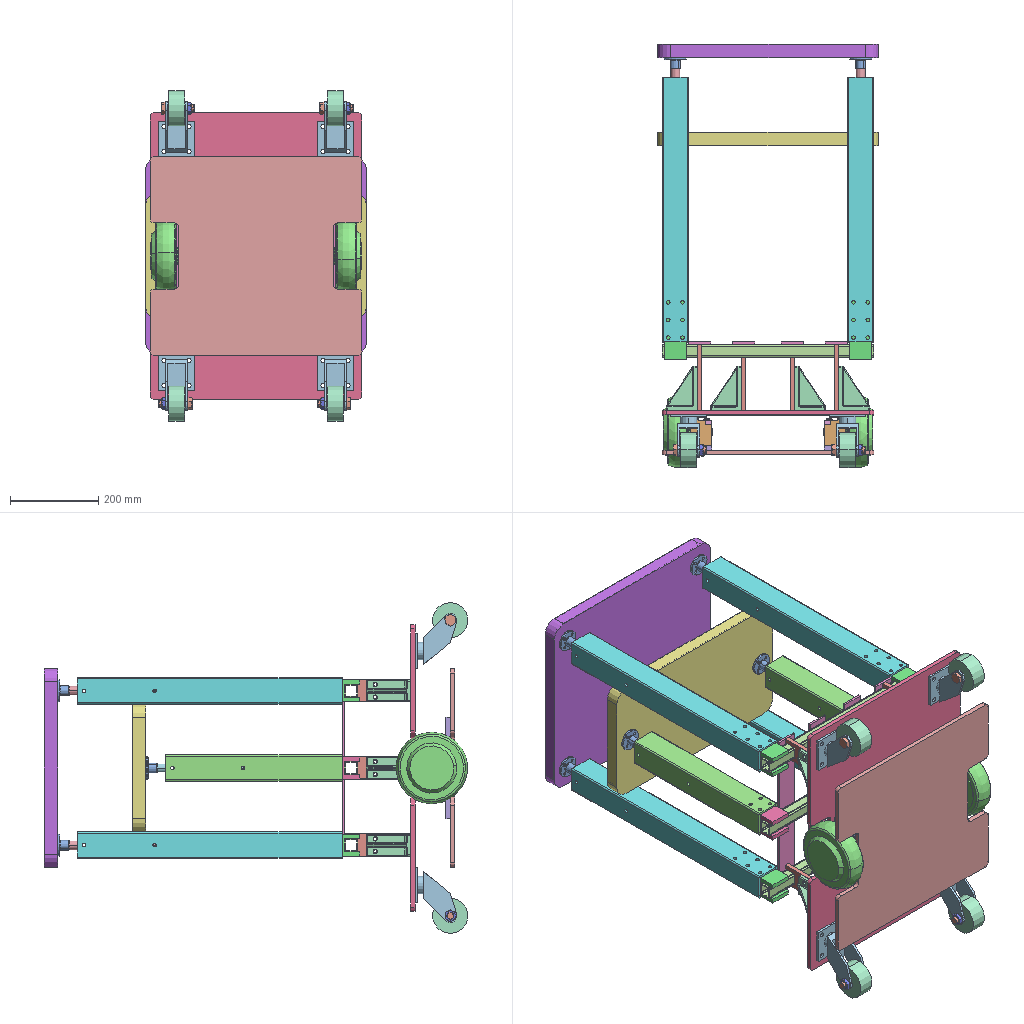Assembly | SolidWorks | 41 different items | 214 placed | box 500 x 959 x 750 mm
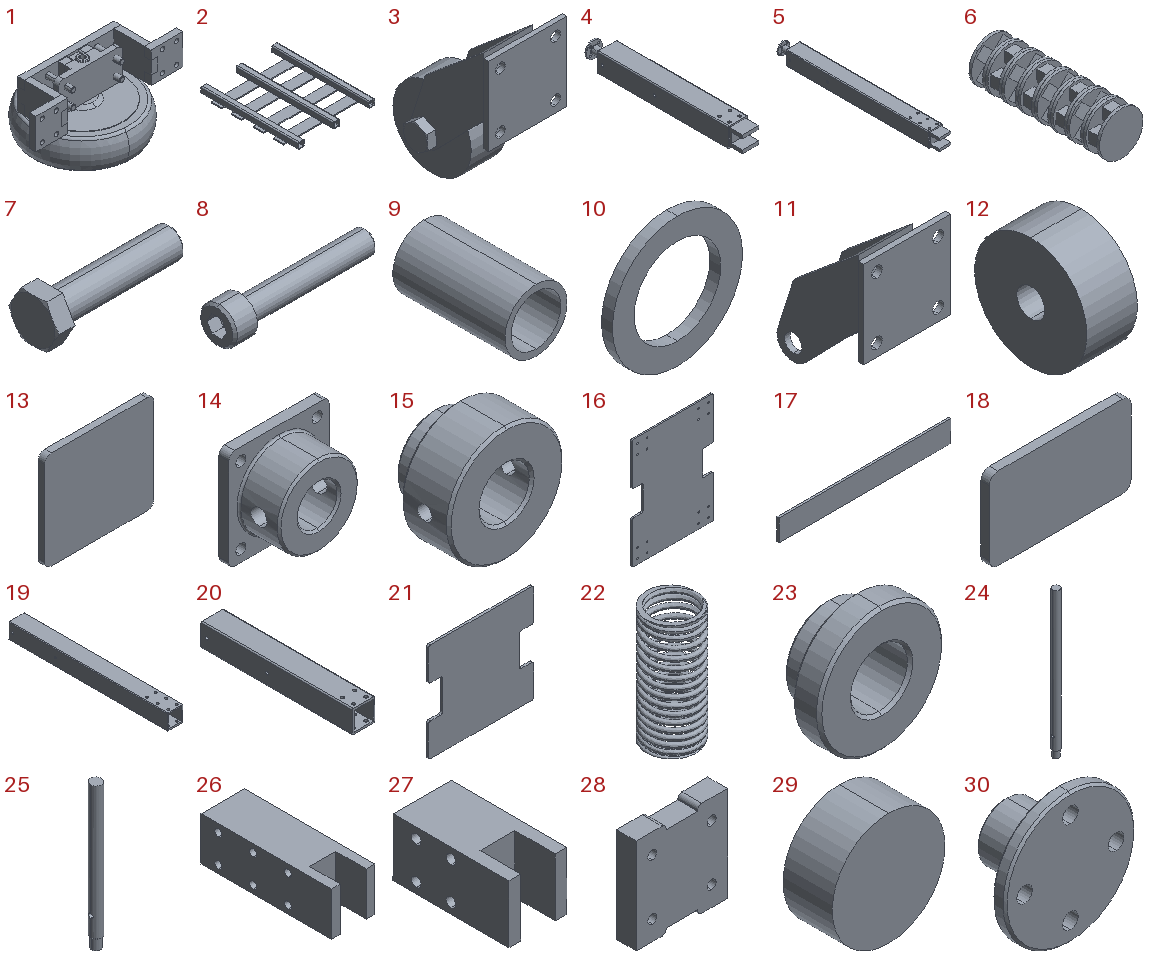Parts list (item | name | quantity | parent item | size | volume | features):
1 | (subassembly) | x2 | - | 230 x 163 x 112 mm | 1242773 mm3 | -
2 | (subassembly) | x1 | - | 400 x 480 x 35 mm | 772823 mm3 | -
3 | (subassembly) | x4 | - | 80 x 120 x 150 mm | 311923 mm3 | features CompositeCurve 1
4 | (subassembly) | x2 | - | 60 x 485 x 60 mm | 1102301 mm3 | -
5 | (subassembly) | x4 | - | 60 x 685 x 60 mm | 1570398 mm3 | -
6 | (subassembly) | x6 | in 4, 5 | 32 x 96 x 32 mm | 42120 mm3 | -
7 | - | x4 | in 3 | 75 x 27.713 x 24 mm | 17960 mm3 | features RevCut 3, Boss 1, Chamfer 1, Extrusion 1, Fillet 1, LPattern 1
8 | - | x8 | in 1 | 53 x 13 x 13 mm | 3161 mm3 | features CirPattern 3, Cut 3, RevCut 2, Fillet 1, LPattern 1, Revolution 1
9 | - | x4 | in 3 | 20 x 36 x 20 mm | 4072 mm3 | features Extrusion 1
10 | - | x8 | in 3 | 24 x 2 x 24 mm | 502.655 mm3 | features Extrusion 1
11 | - | x4 | in 3 | 80 x 95 x 125 mm | 116525 mm3 | features ICE 3, Extrusion 1
12 | - | x4 | in 3 | 36 x 80 x 80 mm | 169646 mm3 | features Revolution 1
13 | - | x1 | - | 500 x 30 x 450 mm | 1262737 mm3 | features Extrusion 1, ICE 1
14 | - | x6 | in 4, 5 | 50 x 25 x 50 mm | 28265 mm3 | features ICE 4, Fillet 2, Chamfer 1, Extrusion 1
15 | - | x6 | in 4, 5 | 48 x 30 x 48 mm | 32861 mm3 | features ICE 3, Chamfer 2, Extrusion 1
16 | - | x1 | - | 480 x 10 x 650 mm | 2911575 mm3 | features Fillet 2, ICE 2, Extrusion 1
17 | - | x4 | in 2 | 400 x 5 x 50 mm | 100000 mm3 | features Extrusion 1
18 | - | x1 | - | 500 x 30 x 290 mm | 838737 mm3 | features Extrusion 1, ICE 1
19 | - | x4 | in 5 | 60 x 600 x 60 mm | 948372 mm3 | features ICE 9, Fillet 2, Extrusion 1
20 | - | x2 | in 4 | 60 x 400 x 60 mm | 650447 mm3 | features ICE 9, Fillet 2, Extrusion 1
21 | - | x1 | - | 480 x 10 x 450 mm | 1964142 mm3 | features Fillet 2, ICE 2, Extrusion 1
22 | - | x6 | in 4, 5 | - | 25238 mm3 | features Helix 1, ICE 1, Sweep 1
23 | - | x6 | in 4, 5 | 46 x 20 x 46 mm | 17526 mm3 | features Chamfer 2, ICE 2, Extrusion 1
24 | - | x4 | in 5 | 20 x 20 x 410 mm | 125504 mm3 | features ICE 4, Chamfer 1, Revolution 1
25 | - | x2 | in 4 | 20 x 20 x 260 mm | 78380 mm3 | features ICE 4, Chamfer 2, Revolution 1
26 | - | x4 | in 5 | 50 x 150 x 50 mm | 308426 mm3 | features ICE 3, Extrusion 1, MirrorPattern 1
27 | - | x2 | in 4 | 50 x 100 x 50 mm | 185436 mm3 | features ICE 4, Extrusion 1
28 | - | x2 | in 1 | 46 x 10 x 48 mm | 19482 mm3 | features ICE 2, Extrusion 1, Fillet 1, HoleWzd 1
29 | - | x6 | in 4, 5 | 32 x 14 x 32 mm | 11259 mm3 | features Extrusion 1
30 | - | x6 | in 4, 5 | 50 x 25 x 50 mm | 12711 mm3 | features ICE 2, Chamfer 1, Extrusion 1, Fillet 1
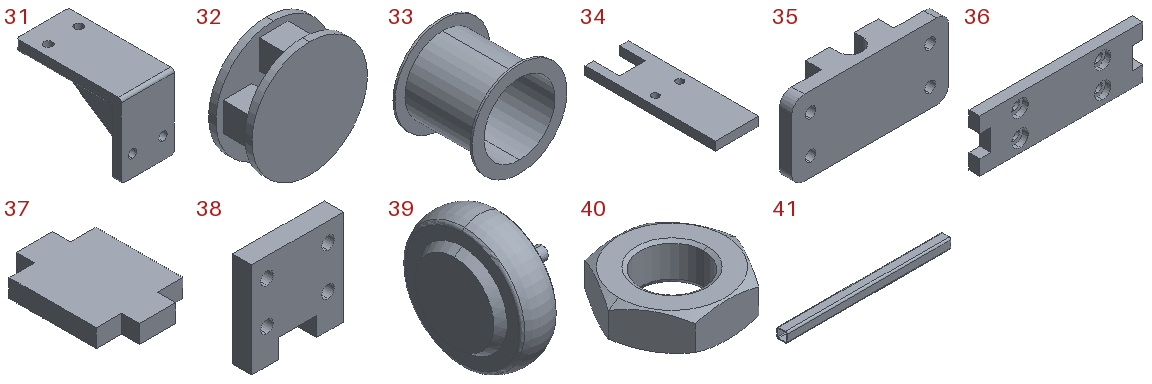31 | - | x6 | - | 50 x 100 x 70 mm | 99196 mm3 | features Fillet 5, ICE 3, MirrorPattern 2, Chamfer 1, Extrusion 1
32 | - | x48 | in 6 | 32 x 12 x 32 mm | 5265 mm3 | features ICE 2, Extrusion 1
33 | - | x18 | in 4, 5 | 48 x 40 x 48 mm | 6000 mm3 | features Revolution 1
34 | - | x6 | - | 50 x 150 x 10 mm | 64995 mm3 | features ICE 2, Extrusion 1
35 | - | x2 | in 1 | 100 x 18 x 48 mm | 49859 mm3 | features HoleWzd 2, ICE 2, Extrusion 1, Fillet 1
36 | - | x2 | in 1 | 150 x 10 x 48 mm | 62310 mm3 | features ICE 2, Extrusion 1, HoleWzd 1
37 | - | x4 | in 1 | 48 x 68 x 10 mm | 27040 mm3 | features Extrusion 1, ICE 1
38 | - | x4 | in 1 | 48 x 10 x 50 mm | 19683 mm3 | features Extrusion 1, HoleWzd 1, ICE 1
39 | - | x2 | in 1 | 112 x 163 x 163 mm | 1005033 mm3 | features ICE 2, Chamfer 1, Fillet 1, Revolution 1
40 | - | x4 | in 3 | 27.713 x 24 x 8 mm | 2715 mm3 | features RevCut 2, Chamfer 1, Extrusion 1, LPattern 1
41 | - | x3 | in 2 | 480 x 30 x 30 mm | 124274 mm3 | features WeldMemberFeat 1, WeldmentFeature 1
Mates (type | each side: item.copy, entity, surface, feature):
In the top assembly
Coincident | 21.1 face plane Boss-Extrude1 | 38.1 face plane Boss-Extrude1
Coincident | 21.1 face plane Boss-Extrude1 | 38.2 face plane Boss-Extrude1
Coincident | 21.1 face plane Boss-Extrude1 | 38.3 face plane Boss-Extrude1
Coincident | 21.1 face plane Boss-Extrude1 | 38.4 face plane Boss-Extrude1
Coincident | 21.1 face plane Boss-Extrude1 | 16.1 face plane Boss-Extrude1
DistanceDim | 16.1 face plane Boss-Extrude1 | 21.1 face plane Boss-Extrude1
Coincident | 16.1 face plane Boss-Extrude1 | 11.1 face plane Boss-Extrude3
DistanceDim | 11.1 face plane Boss-Extrude3 | 16.1 face plane Boss-Extrude1 | 2 times
Coincident | 16.1 face plane Boss-Extrude1 | 11.2 face plane Boss-Extrude3
Coincident | 11.1 face plane Boss-Extrude3 | 11.2 face plane Boss-Extrude3
DistanceDim | 11.2 face plane Boss-Extrude3 | 16.1 face plane Boss-Extrude1
Coincident | 16.1 face plane Boss-Extrude1 | 11.3 face plane Boss-Extrude3
Coincident | 11.2 face plane Boss-Extrude3 | 11.3 face plane Boss-Extrude3
DistanceDim | 11.3 face plane Boss-Extrude3 | 16.1 face plane Boss-Extrude1
Coincident | 16.1 face plane Boss-Extrude1 | 11.4 face plane Boss-Extrude3
Coincident | 11.3 face plane Boss-Extrude3 | 11.4 face plane Boss-Extrude3
Coincident | 11.1 face plane Boss-Extrude3 | 11.4 face plane Boss-Extrude3
Coincident | 16.1 face plane Boss-Extrude1 | assembly face
Parallel | 16.1 face plane Boss-Extrude1 | assembly face | 2 times
DistanceDim | assembly face | 16.1 face plane Boss-Extrude1 | 2 times
Coincident | 41.1 face plane Square tube 30 X 30 X 2.5 | 26.1 face plane Cut-Extrude1 | 2 times
Coincident | 41.1 face plane Square tube 30 X 30 X 2.5 | 26.2 face plane Cut-Extrude1 | 2 times
Coincident | 41.2 face plane Square tube 30 X 30 X 2.5 | 26.3 face plane Cut-Extrude1 | 2 times
Coincident | 41.2 face plane Square tube 30 X 30 X 2.5 | 26.4 face plane Cut-Extrude1 | 2 times
DistanceDim | 26.2 face plane Boss-Extrude2 | 41.1 face plane Square tube 30 X 30 X 2.5
DistanceDim | 26.3 face plane Boss-Extrude2 | 41.2 face plane Square tube 30 X 30 X 2.5
DistanceDim | 26.4 face plane Boss-Extrude2 | 41.2 face plane Square tube 30 X 30 X 2.5
DistanceDim | 26.1 face plane Boss-Extrude2 | 41.1 face plane Square tube 30 X 30 X 2.5
Coincident | 41.3 face plane Square tube 30 X 30 X 2.5 | 27.1 face plane Cut-Extrude2 | 2 times
Coincident | 41.3 face plane Square tube 30 X 30 X 2.5 | 27.2 face plane Cut-Extrude2 | 2 times
DistanceDim | 27.2 face plane Boss-Extrude1 | 41.3 face plane Square tube 30 X 30 X 2.5
DistanceDim | 27.1 face plane Boss-Extrude1 | 41.3 face plane Square tube 30 X 30 X 2.5
Coincident | 19.1 face plane Boss-Extrude1 | 18.1 face plane Boss-Extrude1
Coincident | 30.1 face plane Boss-Extrude2 | 18.1 face plane Boss-Extrude1
DistanceDim | 18.1 face plane Boss-Extrude1 | 19.2 face plane Boss-Extrude1
Coincident | 30.2 face plane Boss-Extrude2 | 13.1 face plane Boss-Extrude1
DistanceDim | 13.1 face plane Boss-Extrude1 | 19.3 face plane Boss-Extrude1 | 2 times
DistanceDim | 21.1 face plane Cut-Extrude2 | 16.1 face plane Boss-Extrude1
Coincident | 21.1 face plane Cut-Extrude1 | 38.3 face plane Boss-Extrude1
Coincident | 21.1 face plane Cut-Extrude1 | 37.1 face plane Boss-Extrude1
Coincident | 21.1 face plane Cut-Extrude1 | 38.1 face plane Boss-Extrude1
Coincident | 21.1 face plane Cut-Extrude1 | 37.2 face plane Boss-Extrude1
Coincident | assembly face | 31.1 face plane Boss-Extrude1 | 2 times
Coincident | assembly face | 31.2 face plane Boss-Extrude1 | 2 times
Coincident | assembly face | 31.3 face plane Boss-Extrude1 | 2 times
Coincident | assembly face | 31.4 face plane Boss-Extrude1 | 2 times
Coincident | assembly face | 31.5 face plane Boss-Extrude1 | 2 times
Coincident | assembly face | 31.6 face plane Boss-Extrude1 | 2 times
Coincident | 31.1 face plane Boss-Extrude1 | 34.1 face plane Boss-Extrude1
Width | 31.1 face plane Boss-Extrude1 | 31.1 face plane Boss-Extrude1 | 34.1 face plane Boss-Extrude1 | 34.1 face plane Boss-Extrude1
Coincident | 16.1 face plane Boss-Extrude1 | 34.1 face plane Boss-Extrude1
Coincident | 31.4 face plane Boss-Extrude1 | 34.2 face plane Boss-Extrude1
Concentric | 31.4 face cylinder Mirror1 | 34.2 face cylinder Cut-Extrude2
Parallel | 31.4 face plane Boss-Extrude1 | 34.2 face plane Boss-Extrude1
Coincident | 31.5 face plane Boss-Extrude1 | 34.3 face plane Boss-Extrude1
Concentric | 31.5 face cylinder Mirror1 | 34.3 face cylinder Cut-Extrude2
Parallel | 31.5 face plane Boss-Extrude1 | 34.3 face plane Boss-Extrude1
Coincident | 31.6 face plane Boss-Extrude1 | 34.4 face plane Boss-Extrude1
Concentric | 31.6 face cylinder Mirror1 | 34.4 face cylinder Cut-Extrude2
Parallel | 31.6 face plane Boss-Extrude1 | 34.4 face plane Boss-Extrude1
Concentric | 31.2 face cylinder Mirror1 | 34.5 face cylinder Cut-Extrude2
Parallel | 31.2 face plane Boss-Extrude1 | 34.5 face plane Boss-Extrude1
Coincident | 31.3 face plane Boss-Extrude1 | 34.6 face plane Boss-Extrude1
Concentric | 31.3 face cylinder Mirror1 | 34.6 face cylinder Cut-Extrude2
Parallel | 31.3 face plane Boss-Extrude1 | 34.6 face plane Boss-Extrude1
In subassembly 4
Coincident | 20.1 face plane Cut-Extrude1 | 14.1 face plane Boss-Extrude3
Concentric | 20.1 face cylinder Cut-Extrude4 | 14.1 face cylinder Cut-Extrude5
Concentric | 20.1 face cylinder Cut-Extrude2 | 14.1 face cylinder Cut-Extrude6
Coincident | 20.1 face plane Cut-Extrude5 | 33.1 face plane Revolve2
Concentric | 20.1 face cylinder Cut-Extrude6 | 33.1 face cylinder Revolve2
Coincident | 20.1 face plane Cut-Extrude5 | 27.3 face plane Boss-Extrude1 | 3 times
Concentric | 14.1 face cylinder Cut-Extrude6 | 25.1 face cylinder Revolve4
Concentric | 20.1 face cylinder Cut-Extrude4 | 25.1 face cylinder Cut-Extrude1
DistanceDim | 23.1 face plane Boss-Extrude1 | 15.1 face plane Boss-Extrude1
Coincident | 22.1 face plane Cut-Extrude1 | 23.1 face plane Boss-Extrude1
Concentric | 33.1 face cylinder Revolve2 | 33.2 face cylinder Revolve2
Coincident | 33.1 face plane Revolve2 | 33.2 face plane Revolve2
Concentric | 25.1 face cylinder Revolve4 | 33.3 face cylinder Revolve2
Coincident | 33.2 face plane Revolve2 | 33.3 face plane Revolve2
Coincident | 25.1 face plane Boss-Extrude3 | 32.1 face plane Boss-Extrude8
Concentric | 25.1 face cylinder Revolve4 | 32.1 face cylinder Boss-Extrude8
Parallel | 27.3 face plane Boss-Extrude1 | 32.2 face plane Boss-Extrude7
Concentric | 23.1 face cylinder Boss-Extrude1 | 15.1 face cylinder Boss-Extrude1
Concentric | 25.1 face cylinder Revolve4 | 15.1 face cylinder Cut-Extrude3
Concentric | 20.1 face cylinder Cut-Extrude7 | 15.1 face cylinder Cut-Extrude2
Concentric | 25.1 face cylinder Boss-Extrude5 | 30.3 face cylinder Boss-Extrude3
Coincident | 25.1 face plane Boss-Extrude4 | 30.3 face plane Boss-Extrude3
Coincident | 27.3 face plane Cut-Extrude3 | 29.1 face plane Boss-Extrude1
Concentric | 27.3 face cylinder Cut-Extrude3 | 29.1 face cylinder Boss-Extrude1
In subassembly 6
Coincident | 32.3 face plane Boss-Extrude8 | 32.4 face plane Boss-Extrude2
Concentric | 32.3 face cylinder Boss-Extrude8 | 32.4 face cylinder Boss-Extrude2
Concentric | 32.3 face cylinder Boss-Extrude8 | 32.5 face cylinder Boss-Extrude2
Coincident | 32.4 face plane Boss-Extrude8 | 32.5 face plane Boss-Extrude2
Coincident | 32.6 face plane Boss-Extrude2 | 32.5 face plane Boss-Extrude8
Concentric | 32.6 face cylinder Boss-Extrude2 | 32.5 face cylinder Boss-Extrude8
Coincident | 32.7 face plane Boss-Extrude8 | 32.8 face plane Boss-Extrude2
Concentric | 32.7 face cylinder Boss-Extrude8 | 32.8 face cylinder Boss-Extrude2
Coincident | 32.7 face plane Boss-Extrude2 | 32.6 face plane Boss-Extrude8
Concentric | 32.7 face cylinder Boss-Extrude2 | 32.6 face cylinder Boss-Extrude8
Coincident | 32.9 face plane Boss-Extrude2 | 32.10 face plane Boss-Extrude8 | 2 times
Concentric | 32.9 face cylinder Boss-Extrude2 | 32.10 face cylinder Boss-Extrude8
Coincident | 32.10 face plane Boss-Extrude2 | 32.8 face plane Boss-Extrude8
Concentric | 32.10 face cylinder Boss-Extrude2 | 32.8 face cylinder Boss-Extrude8
PlanarAngleDim | 32.4 face plane Boss-Extrude7 | 32.3 face plane Boss-Extrude7
Coincident | 32.3 face plane Boss-Extrude7 | 32.5 face plane Boss-Extrude7
Coincident | 32.7 face plane Boss-Extrude7 | 32.5 face plane Boss-Extrude7
Coincident | 32.4 face plane Boss-Extrude7 | 32.6 face plane Boss-Extrude7
Coincident | 32.6 face plane Boss-Extrude7 | 32.8 face plane Boss-Extrude7
Coincident | 32.10 face plane Boss-Extrude7 | 32.7 face plane Boss-Extrude7
Coincident | 32.9 face plane Boss-Extrude7 | 32.8 face plane Boss-Extrude7
In subassembly 3
Concentric | 9.1 face cylinder Boss-Extrude1 | 12.1 face cylinder Revolve1
Coincident | 9.1 face plane Boss-Extrude1 | 12.1 face plane Revolve1
Coincident | 10.1 edge | 12.1 face plane Revolve1
Concentric | 9.1 face cylinder Boss-Extrude1 | 10.1 face cylinder Boss-Extrude3
Coincident | 10.2 face plane Boss-Extrude3 | 12.1 face plane Revolve1
Concentric | 9.1 face cylinder Boss-Extrude1 | 10.2 face cylinder Boss-Extrude3
Concentric | 11.5 face cylinder Boss-Extrude6 | 9.1 face cylinder Boss-Extrude1
Coincident | 11.5 face plane Cut-Extrude1 | 10.1 face plane Boss-Extrude3
Concentric | 9.1 face cylinder Boss-Extrude1 | 7.1 face cylinder BaseBody
Coincident | 11.5 face plane Boss-Extrude6 | 7.1 face plane BaseHead
Concentric | 7.1 face cylinder BaseBody | 40.1 face cylinder BaseNut
Coincident | 11.5 face plane Boss-Extrude6 | 40.1 face plane BaseNut
In subassembly 5
Concentric | 19.4 face cylinder Cut-Extrude7 | 14.1 face cylinder Cut-Extrude6
Concentric | 19.4 face cylinder Cut-Extrude3 | 14.1 face cylinder Cut-Extrude5
Concentric | 19.4 face cylinder Cut-Extrude6 | 33.1 face cylinder Revolve2
Coincident | 19.4 face plane Cut-Extrude5 | 33.1 face plane Revolve2
Coincident | 19.4 face plane Cut-Extrude5 | 26.5 face plane Boss-Extrude2 | 3 times
Coincident | 19.4 face plane Cut-Extrude5 | 26.5 select_type:24
Concentric | 14.1 face cylinder Cut-Extrude6 | 24.1 face cylinder Revolve4
Concentric | 19.4 face cylinder Cut-Extrude3 | 24.1 face cylinder Cut-Extrude1
Concentric | 15.1 face cylinder Cut-Extrude3 | 23.1 face cylinder Cut-Extrude1
Coincident | 22.2 face plane Cut-Extrude1 | 23.1 face plane Boss-Extrude1
Coincident | 22.2 face plane Cut-Extrude1 | 15.1 face plane Boss-Extrude1
Concentric | 24.1 face cylinder Boss-Extrude2 | 30.3 face cylinder Boss-Extrude3
Coincident | 24.1 face plane Boss-Extrude1 | 30.3 face plane Boss-Extrude3
Concentric | 19.4 face cylinder Cut-Extrude8 | 15.1 face cylinder Cut-Extrude2
Concentric | 24.1 face cylinder Revolve4 | 23.1 face cylinder Cut-Extrude1
Coincident | 33.2 face plane Revolve2 | 33.3 face plane Revolve2
Concentric | 33.2 face cylinder Revolve2 | 33.3 face cylinder Revolve2
Concentric | 33.1 face cylinder Revolve2 | 33.2 face cylinder Revolve2
Coincident | 33.1 face plane Revolve2 | 33.2 face plane Revolve2
Coincident | 24.1 face plane Boss-Extrude4 | 32.1 face plane Boss-Extrude8
Concentric | 24.1 face cylinder Revolve4 | 32.1 face cylinder Boss-Extrude8
Parallel | 26.5 face plane Boss-Extrude2 | 32.11 face plane Boss-Extrude7
Coincident | 26.5 face plane Cut-Extrude2 | 29.1 face plane Boss-Extrude1
Concentric | 26.5 face cylinder Cut-Extrude2 | 29.1 face cylinder Boss-Extrude1
In subassembly 2
Width | 2.1 face | 2.1 face | 41.4 face plane Square tube 30 X 30 X 2.5 | 41.4 face plane Square tube 30 X 30 X 2.5
DistanceDim | 41.4 face plane Square tube 30 X 30 X 2.5 | 2.1 face
Coincident | 41.4 face plane Square tube 30 X 30 X 2.5 | 2.1 face
DistanceDim | 41.4 face plane Square tube 30 X 30 X 2.5 | 17.1 face plane Boss-Extrude1
Coincident | 41.4 face plane Square tube 30 X 30 X 2.5 | 17.1 face plane Boss-Extrude1
DistanceDim | 41.5 face plane Square tube 30 X 30 X 2.5 | 17.1 face plane Boss-Extrude1
Coincident | 17.1 face plane Boss-Extrude1 | 41.5 face plane Square tube 30 X 30 X 2.5
DistanceDim | 41.6 face plane Square tube 30 X 30 X 2.5 | 41.4 face plane Square tube 30 X 30 X 2.5
Coincident | 41.6 face plane Square tube 30 X 30 X 2.5 | 17.2 face plane Boss-Extrude1 | 2 times
Coincident | 17.1 face plane Boss-Extrude1 | 41.6 face plane Square tube 30 X 30 X 2.5
DistanceDim | 17.1 face plane Boss-Extrude1 | 41.6 face plane Square tube 30 X 30 X 2.5
DistanceDim | 17.3 face plane Boss-Extrude1 | 41.5 face plane Square tube 30 X 30 X 2.5
Coincident | 41.6 face plane Square tube 30 X 30 X 2.5 | 17.4 face plane Boss-Extrude1
DistanceDim | 17.4 face plane Boss-Extrude1 | 17.3 face plane Boss-Extrude1
DistanceDim | 17.4 face plane Boss-Extrude1 | 17.2 face plane Boss-Extrude1
In subassembly 1
Coincident | 35.1 face plane Boss-Extrude2 | 28.1 face plane Boss-Extrude1 | 2 times
Coincident | 35.1 face plane Boss-Extrude1 | 28.1 face plane Boss-Extrude1
Width | 36.1 face plane Boss-Extrude1 | 36.1 face plane Boss-Extrude1 | 35.1 face plane Boss-Extrude1 | 35.1 face plane Boss-Extrude1 | 2 times
Concentric | 36.1 face cylinder CBORE for M8 Cheese Head Screw1 | 1.1 face
LimitDistanceDim | 36.1 face plane Boss-Extrude1 | 28.1 face plane Boss-Extrude1
Concentric | 36.1 face cone CBORE for M8 Cheese Head Screw1 | 8.1 face cylinder Base-Revolve
Concentric | 36.1 face cone CBORE for M8 Cheese Head Screw1 | 8.2 face cylinder Base-Revolve
Concentric | 36.1 face cone CBORE for M8 Cheese Head Screw1 | 8.3 face cylinder Base-Revolve
Concentric | 36.1 face cylinder CBORE for M8 Cheese Head Screw1 | 8.4 face cylinder Base-Revolve
Coincident | 8.4 face plane Base-Revolve | 8.2 face plane Base-Revolve
Coincident | 8.4 face plane Base-Revolve | 8.3 face plane Base-Revolve
Coincident | 36.1 face plane Boss-Extrude1 | 37.3 face plane Boss-Extrude1 | 3 times
Coincident | 36.1 face plane Boss-Extrude1 | 37.4 face plane Boss-Extrude1 | 2 times
Coincident | 36.1 edge | 37.4 face plane Boss-Extrude1
Coincident | 37.3 face plane Boss-Extrude1 | 38.5 face plane Boss-Extrude1 | 3 times
Coincident | 37.4 face plane Cut-Extrude1 | 38.6 face plane Boss-Extrude1
Coincident | 37.4 face plane Boss-Extrude1 | 38.6 face plane Boss-Extrude1 | 2 times
Concentric | 35.1 face cylinder Cut-Extrude1 | 39.1 face cylinder Revolve1
DistanceDim | 39.1 face plane Cut-Extrude2 | 28.1 face plane Cut-Extrude1
Coincident | 36.1 face plane CBORE for M8 Cheese Head Screw1 | 8.1 face plane Base-Revolve
Coincident | 36.1 face plane CBORE for M8 Cheese Head Screw1 | 8.4 face plane Base-Revolve